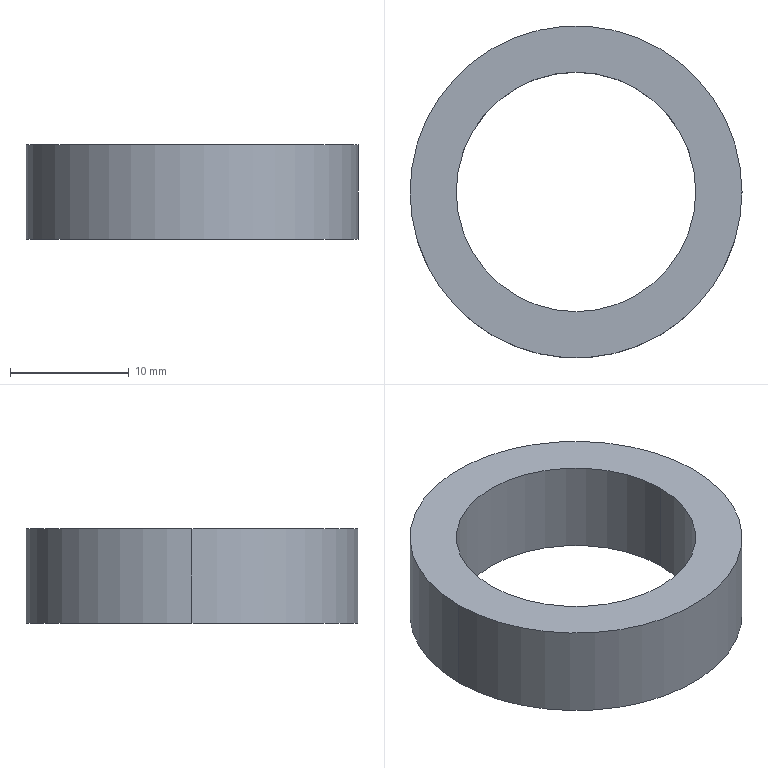Part | SolidWorks | features Extrusion 1 | 1 solid | 6 faces | box 28 x 28 x 8 mm | volume 2362 mm3 | cylinder 4 | plane 2 | commonest cylinder face diameters 20.2 x2 28 x2
STEP:
#1=CARTESIAN_POINT('',(-10.1,0.,8.));
#2=VERTEX_POINT('',#1);
#3=CARTESIAN_POINT('',(10.1,0.,8.));
#4=VERTEX_POINT('',#3);
#5=CARTESIAN_POINT('',(0.,0.,8.));
#6=DIRECTION('',(0.,0.,1.));
#7=DIRECTION('',(1.,0.,0.));
#8=AXIS2_PLACEMENT_3D('',#5,#6,#7);
#9=CIRCLE('',#8,10.1);
#10=EDGE_CURVE('',#2,#4,#9,.T.);
#11=ORIENTED_EDGE('',*,*,#10,.T.);
#12=CARTESIAN_POINT('',(10.1,0.,0.));
#13=VERTEX_POINT('',#12);
#14=CARTESIAN_POINT('',(10.1,0.,8.));
#15=DIRECTION('',(0.,0.,-1.));
#16=VECTOR('',#15,1000.);
#17=LINE('',#14,#16);
#18=EDGE_CURVE('',#4,#13,#17,.T.);
#19=ORIENTED_EDGE('',*,*,#18,.T.);
#20=CARTESIAN_POINT('',(-10.1,0.,0.));
#21=VERTEX_POINT('',#20);
#22=CARTESIAN_POINT('',(0.,0.,0.));
#23=DIRECTION('',(0.,0.,1.));
#24=DIRECTION('',(1.,0.,0.));
#25=AXIS2_PLACEMENT_3D('',#22,#23,#24);
#26=CIRCLE('',#25,10.1);
#27=EDGE_CURVE('',#21,#13,#26,.T.);
#28=ORIENTED_EDGE('',*,*,#27,.F.);
#29=CARTESIAN_POINT('',(-10.1,0.,8.));
#30=DIRECTION('',(0.,0.,-1.));
#31=VECTOR('',#30,1000.);
#32=LINE('',#29,#31);
#33=EDGE_CURVE('',#2,#21,#32,.T.);
#34=ORIENTED_EDGE('',*,*,#33,.F.);
#35=EDGE_LOOP('',(#11,#19,#28,#34));
#36=FACE_OUTER_BOUND('',#35,.T.);
#37=CARTESIAN_POINT('',(0.,0.,8.));
#38=DIRECTION('',(0.,0.,-1.));
#39=DIRECTION('',(-1.,0.,0.));
#40=AXIS2_PLACEMENT_3D('',#37,#38,#39);
#41=CYLINDRICAL_SURFACE('',#40,10.1);
#42=ADVANCED_FACE('',(#36),#41,.F.);
#43=CARTESIAN_POINT('',(14.,0.,8.));
#44=VERTEX_POINT('',#43);
#45=CARTESIAN_POINT('',(-14.,0.,8.));
#46=VERTEX_POINT('',#45);
#47=CARTESIAN_POINT('',(0.,0.,8.));
#48=DIRECTION('',(0.,0.,1.));
#49=DIRECTION('',(1.,0.,0.));
#50=AXIS2_PLACEMENT_3D('',#47,#48,#49);
#51=CIRCLE('',#50,14.);
#52=EDGE_CURVE('',#44,#46,#51,.T.);
#53=ORIENTED_EDGE('',*,*,#52,.F.);
#54=CARTESIAN_POINT('',(14.,0.,0.));
#55=VERTEX_POINT('',#54);
#56=CARTESIAN_POINT('',(14.,0.,8.));
#57=DIRECTION('',(0.,0.,-1.));
#58=VECTOR('',#57,1000.);
#59=LINE('',#56,#58);
#60=EDGE_CURVE('',#44,#55,#59,.T.);
#61=ORIENTED_EDGE('',*,*,#60,.T.);
#62=CARTESIAN_POINT('',(-14.,0.,0.));
#63=VERTEX_POINT('',#62);
#64=CARTESIAN_POINT('',(0.,0.,0.));
#65=DIRECTION('',(0.,0.,1.));
#66=DIRECTION('',(1.,0.,0.));
#67=AXIS2_PLACEMENT_3D('',#64,#65,#66);
#68=CIRCLE('',#67,14.);
#69=EDGE_CURVE('',#55,#63,#68,.T.);
#70=ORIENTED_EDGE('',*,*,#69,.T.);
#71=CARTESIAN_POINT('',(-14.,0.,8.));
#72=DIRECTION('',(0.,0.,-1.));
#73=VECTOR('',#72,1000.);
#74=LINE('',#71,#73);
#75=EDGE_CURVE('',#46,#63,#74,.T.);
#76=ORIENTED_EDGE('',*,*,#75,.F.);
#77=EDGE_LOOP('',(#53,#61,#70,#76));
#78=FACE_OUTER_BOUND('',#77,.T.);
#79=CARTESIAN_POINT('',(0.,0.,8.));
#80=DIRECTION('',(0.,0.,-1.));
#81=DIRECTION('',(-1.,0.,0.));
#82=AXIS2_PLACEMENT_3D('',#79,#80,#81);
#83=CYLINDRICAL_SURFACE('',#82,14.);
#84=ADVANCED_FACE('',(#78),#83,.T.);
#85=CARTESIAN_POINT('',(0.,0.,8.));
#86=DIRECTION('',(0.,0.,1.));
#87=DIRECTION('',(1.,0.,0.));
#88=AXIS2_PLACEMENT_3D('',#85,#86,#87);
#89=CIRCLE('',#88,14.);
#90=EDGE_CURVE('',#46,#44,#89,.T.);
#91=ORIENTED_EDGE('',*,*,#90,.T.);
#92=ORIENTED_EDGE('',*,*,#52,.T.);
#93=EDGE_LOOP('',(#91,#92));
#94=FACE_OUTER_BOUND('',#93,.T.);
#95=ORIENTED_EDGE('',*,*,#10,.F.);
#96=CARTESIAN_POINT('',(0.,0.,8.));
#97=DIRECTION('',(0.,0.,1.));
#98=DIRECTION('',(1.,0.,0.));
#99=AXIS2_PLACEMENT_3D('',#96,#97,#98);
#100=CIRCLE('',#99,10.1);
#101=EDGE_CURVE('',#4,#2,#100,.T.);
#102=ORIENTED_EDGE('',*,*,#101,.F.);
#103=EDGE_LOOP('',(#95,#102));
#104=FACE_BOUND('',#103,.T.);
#105=CARTESIAN_POINT('',(0.,0.,8.));
#106=DIRECTION('',(0.,0.,1.));
#107=DIRECTION('',(1.,0.,0.));
#108=AXIS2_PLACEMENT_3D('',#105,#106,#107);
#109=PLANE('',#108);
#110=ADVANCED_FACE('',(#94,#104),#109,.T.);
#111=CARTESIAN_POINT('',(0.,0.,0.));
#112=DIRECTION('',(0.,0.,1.));
#113=DIRECTION('',(1.,0.,0.));
#114=AXIS2_PLACEMENT_3D('',#111,#112,#113);
#115=CIRCLE('',#114,14.);
#116=EDGE_CURVE('',#63,#55,#115,.T.);
#117=ORIENTED_EDGE('',*,*,#116,.F.);
#118=ORIENTED_EDGE('',*,*,#69,.F.);
#119=EDGE_LOOP('',(#117,#118));
#120=FACE_OUTER_BOUND('',#119,.T.);
#121=ORIENTED_EDGE('',*,*,#27,.T.);
#122=CARTESIAN_POINT('',(0.,0.,0.));
#123=DIRECTION('',(0.,0.,1.));
#124=DIRECTION('',(1.,0.,0.));
#125=AXIS2_PLACEMENT_3D('',#122,#123,#124);
#126=CIRCLE('',#125,10.1);
#127=EDGE_CURVE('',#13,#21,#126,.T.);
#128=ORIENTED_EDGE('',*,*,#127,.T.);
#129=EDGE_LOOP('',(#121,#128));
#130=FACE_BOUND('',#129,.T.);
#131=CARTESIAN_POINT('',(0.,0.,0.));
#132=DIRECTION('',(0.,0.,1.));
#133=DIRECTION('',(1.,0.,0.));
#134=AXIS2_PLACEMENT_3D('',#131,#132,#133);
#135=PLANE('',#134);
#136=ADVANCED_FACE('',(#120,#130),#135,.F.);
#137=ORIENTED_EDGE('',*,*,#60,.F.);
#138=ORIENTED_EDGE('',*,*,#90,.F.);
#139=ORIENTED_EDGE('',*,*,#75,.T.);
#140=ORIENTED_EDGE('',*,*,#116,.T.);
#141=EDGE_LOOP('',(#137,#138,#139,#140));
#142=FACE_OUTER_BOUND('',#141,.T.);
#143=CARTESIAN_POINT('',(0.,0.,8.));
#144=DIRECTION('',(0.,0.,-1.));
#145=DIRECTION('',(-1.,0.,0.));
#146=AXIS2_PLACEMENT_3D('',#143,#144,#145);
#147=CYLINDRICAL_SURFACE('',#146,14.);
#148=ADVANCED_FACE('',(#142),#147,.T.);
#149=ORIENTED_EDGE('',*,*,#18,.F.);
#150=ORIENTED_EDGE('',*,*,#101,.T.);
#151=ORIENTED_EDGE('',*,*,#33,.T.);
#152=ORIENTED_EDGE('',*,*,#127,.F.);
#153=EDGE_LOOP('',(#149,#150,#151,#152));
#154=FACE_OUTER_BOUND('',#153,.T.);
#155=CARTESIAN_POINT('',(0.,0.,8.));
#156=DIRECTION('',(0.,0.,-1.));
#157=DIRECTION('',(-1.,0.,0.));
#158=AXIS2_PLACEMENT_3D('',#155,#156,#157);
#159=CYLINDRICAL_SURFACE('',#158,10.1);
#160=ADVANCED_FACE('',(#154),#159,.F.);
#161=CLOSED_SHELL('',(#42,#84,#110,#136,#148,#160));
#162=MANIFOLD_SOLID_BREP('',#161);
#163=CARTESIAN_POINT('',(0.,0.,0.));
#164=DIRECTION('',(0.,0.,1.));
#165=DIRECTION('',(1.,0.,0.));
#166=AXIS2_PLACEMENT_3D('',#163,#164,#165);
#167=(LENGTH_UNIT()NAMED_UNIT(*)SI_UNIT(.MILLI.,.METRE.));
#168=UNCERTAINTY_MEASURE_WITH_UNIT(LENGTH_MEASURE(0.00001),#167,'','');
#169=(NAMED_UNIT(*)PLANE_ANGLE_UNIT()SI_UNIT($,.RADIAN.));
#170=(NAMED_UNIT(*)SI_UNIT($,.STERADIAN.)SOLID_ANGLE_UNIT());
#171=(GEOMETRIC_REPRESENTATION_CONTEXT(3)GLOBAL_UNCERTAINTY_ASSIGNED_CONTEXT((#168))GLOBAL_UNIT_ASSIGNED_CONTEXT((#167,#169,#170))REPRESENTATION_CONTEXT('',''));
#172=ADVANCED_BREP_SHAPE_REPRESENTATION('',(#162,#166),#171);